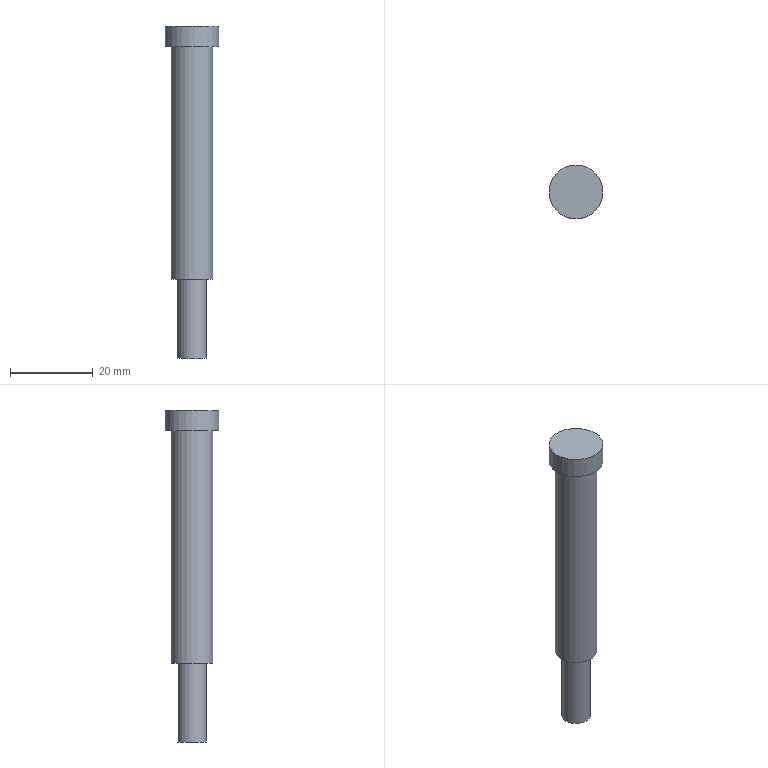Part | NX | features solid 2 | 1 solid | 7 faces | box 13 x 13 x 80 mm | volume 5793 mm3 | plane 4 | cylinder 3 | commonest cylinder face diameters 7 x1 10 x1 13 x1
STEP:
#1=CARTESIAN_POINT('',(439.131,-6.613,119.));
#2=VERTEX_POINT('',#1);
#3=CARTESIAN_POINT('',(434.131,-6.613,119.));
#4=DIRECTION('',(0.,0.,1.));
#5=DIRECTION('',(1.,0.,0.));
#6=AXIS2_PLACEMENT_3D('',#3,#4,#5);
#7=CIRCLE('',#6,5.);
#8=EDGE_CURVE('',#2,#2,#7,.T.);
#9=ORIENTED_EDGE('',*,*,#8,.T.);
#10=EDGE_LOOP('',(#9));
#11=FACE_BOUND('',#10,.T.);
#12=CARTESIAN_POINT('',(439.131,-6.613,175.));
#13=VERTEX_POINT('',#12);
#14=CARTESIAN_POINT('',(434.131,-6.613,175.));
#15=DIRECTION('',(0.,0.,1.));
#16=DIRECTION('',(1.,0.,0.));
#17=AXIS2_PLACEMENT_3D('',#14,#15,#16);
#18=CIRCLE('',#17,5.);
#19=EDGE_CURVE('',#13,#13,#18,.T.);
#20=ORIENTED_EDGE('',*,*,#19,.F.);
#21=EDGE_LOOP('',(#20));
#22=FACE_BOUND('',#21,.T.);
#23=CARTESIAN_POINT('',(434.131,-6.613,180.));
#24=DIRECTION('',(0.,0.,-1.));
#25=DIRECTION('',(-1.,0.,0.));
#26=AXIS2_PLACEMENT_3D('',#23,#24,#25);
#27=CYLINDRICAL_SURFACE('',#26,5.);
#28=ADVANCED_FACE('',(#11,#22),#27,.T.);
#29=CARTESIAN_POINT('',(437.631,-6.613,119.));
#30=VERTEX_POINT('',#29);
#31=CARTESIAN_POINT('',(434.131,-6.613,119.));
#32=DIRECTION('',(0.,0.,1.));
#33=DIRECTION('',(1.,0.,0.));
#34=AXIS2_PLACEMENT_3D('',#31,#32,#33);
#35=CIRCLE('',#34,3.5);
#36=EDGE_CURVE('',#30,#30,#35,.T.);
#37=ORIENTED_EDGE('',*,*,#36,.T.);
#38=EDGE_LOOP('',(#37));
#39=FACE_BOUND('',#38,.T.);
#40=ORIENTED_EDGE('',*,*,#8,.F.);
#41=EDGE_LOOP('',(#40));
#42=FACE_BOUND('',#41,.T.);
#43=CARTESIAN_POINT('',(434.131,-6.613,119.));
#44=DIRECTION('',(0.,0.,1.));
#45=DIRECTION('',(1.,0.,0.));
#46=AXIS2_PLACEMENT_3D('',#43,#44,#45);
#47=PLANE('',#46);
#48=ADVANCED_FACE('',(#39,#42),#47,.F.);
#49=CARTESIAN_POINT('',(440.631,-6.613,175.));
#50=VERTEX_POINT('',#49);
#51=CARTESIAN_POINT('',(434.131,-6.613,175.));
#52=DIRECTION('',(0.,0.,1.));
#53=DIRECTION('',(1.,0.,0.));
#54=AXIS2_PLACEMENT_3D('',#51,#52,#53);
#55=CIRCLE('',#54,6.5);
#56=EDGE_CURVE('',#50,#50,#55,.T.);
#57=ORIENTED_EDGE('',*,*,#56,.F.);
#58=EDGE_LOOP('',(#57));
#59=FACE_BOUND('',#58,.T.);
#60=ORIENTED_EDGE('',*,*,#19,.T.);
#61=EDGE_LOOP('',(#60));
#62=FACE_BOUND('',#61,.T.);
#63=CARTESIAN_POINT('',(434.131,-6.613,175.));
#64=DIRECTION('',(0.,0.,1.));
#65=DIRECTION('',(1.,0.,0.));
#66=AXIS2_PLACEMENT_3D('',#63,#64,#65);
#67=PLANE('',#66);
#68=ADVANCED_FACE('',(#59,#62),#67,.F.);
#69=ORIENTED_EDGE('',*,*,#56,.T.);
#70=EDGE_LOOP('',(#69));
#71=FACE_BOUND('',#70,.T.);
#72=CARTESIAN_POINT('',(440.631,-6.613,180.));
#73=VERTEX_POINT('',#72);
#74=CARTESIAN_POINT('',(434.131,-6.613,180.));
#75=DIRECTION('',(0.,0.,1.));
#76=DIRECTION('',(1.,0.,0.));
#77=AXIS2_PLACEMENT_3D('',#74,#75,#76);
#78=CIRCLE('',#77,6.5);
#79=EDGE_CURVE('',#73,#73,#78,.T.);
#80=ORIENTED_EDGE('',*,*,#79,.F.);
#81=EDGE_LOOP('',(#80));
#82=FACE_BOUND('',#81,.T.);
#83=CARTESIAN_POINT('',(434.131,-6.613,175.));
#84=DIRECTION('',(0.,0.,1.));
#85=DIRECTION('',(1.,0.,0.));
#86=AXIS2_PLACEMENT_3D('',#83,#84,#85);
#87=CYLINDRICAL_SURFACE('',#86,6.5);
#88=ADVANCED_FACE('',(#71,#82),#87,.T.);
#89=ORIENTED_EDGE('',*,*,#79,.T.);
#90=EDGE_LOOP('',(#89));
#91=FACE_BOUND('',#90,.T.);
#92=CARTESIAN_POINT('',(434.131,-6.613,180.));
#93=DIRECTION('',(0.,0.,1.));
#94=DIRECTION('',(1.,0.,0.));
#95=AXIS2_PLACEMENT_3D('',#92,#93,#94);
#96=PLANE('',#95);
#97=ADVANCED_FACE('',(#91),#96,.T.);
#98=CARTESIAN_POINT('',(437.631,-6.613,100.));
#99=VERTEX_POINT('',#98);
#100=CARTESIAN_POINT('',(434.131,-6.613,100.));
#101=DIRECTION('',(0.,0.,1.));
#102=DIRECTION('',(1.,0.,0.));
#103=AXIS2_PLACEMENT_3D('',#100,#101,#102);
#104=CIRCLE('',#103,3.5);
#105=EDGE_CURVE('',#99,#99,#104,.T.);
#106=ORIENTED_EDGE('',*,*,#105,.T.);
#107=EDGE_LOOP('',(#106));
#108=FACE_BOUND('',#107,.T.);
#109=ORIENTED_EDGE('',*,*,#36,.F.);
#110=EDGE_LOOP('',(#109));
#111=FACE_BOUND('',#110,.T.);
#112=CARTESIAN_POINT('',(434.131,-6.613,100.));
#113=DIRECTION('',(0.,0.,1.));
#114=DIRECTION('',(1.,0.,0.));
#115=AXIS2_PLACEMENT_3D('',#112,#113,#114);
#116=CYLINDRICAL_SURFACE('',#115,3.5);
#117=ADVANCED_FACE('',(#108,#111),#116,.T.);
#118=ORIENTED_EDGE('',*,*,#105,.F.);
#119=EDGE_LOOP('',(#118));
#120=FACE_BOUND('',#119,.T.);
#121=CARTESIAN_POINT('',(434.131,-6.613,100.));
#122=DIRECTION('',(0.,0.,1.));
#123=DIRECTION('',(1.,0.,0.));
#124=AXIS2_PLACEMENT_3D('',#121,#122,#123);
#125=PLANE('',#124);
#126=ADVANCED_FACE('',(#120),#125,.F.);
#127=CLOSED_SHELL('',(#28,#48,#68,#88,#97,#117,#126));
#128=MANIFOLD_SOLID_BREP('',#127);
#129=(LENGTH_UNIT()NAMED_UNIT(*)SI_UNIT(.MILLI.,.METRE.));
#130=UNCERTAINTY_MEASURE_WITH_UNIT(LENGTH_MEASURE(0.00001),#129,'','');
#131=(NAMED_UNIT(*)PLANE_ANGLE_UNIT()SI_UNIT($,.RADIAN.));
#132=(NAMED_UNIT(*)SI_UNIT($,.STERADIAN.)SOLID_ANGLE_UNIT());
#133=(GEOMETRIC_REPRESENTATION_CONTEXT(3)GLOBAL_UNCERTAINTY_ASSIGNED_CONTEXT((#130))GLOBAL_UNIT_ASSIGNED_CONTEXT((#129,#131,#132))REPRESENTATION_CONTEXT('',''));
#134=ADVANCED_BREP_SHAPE_REPRESENTATION('',(#128),#133);